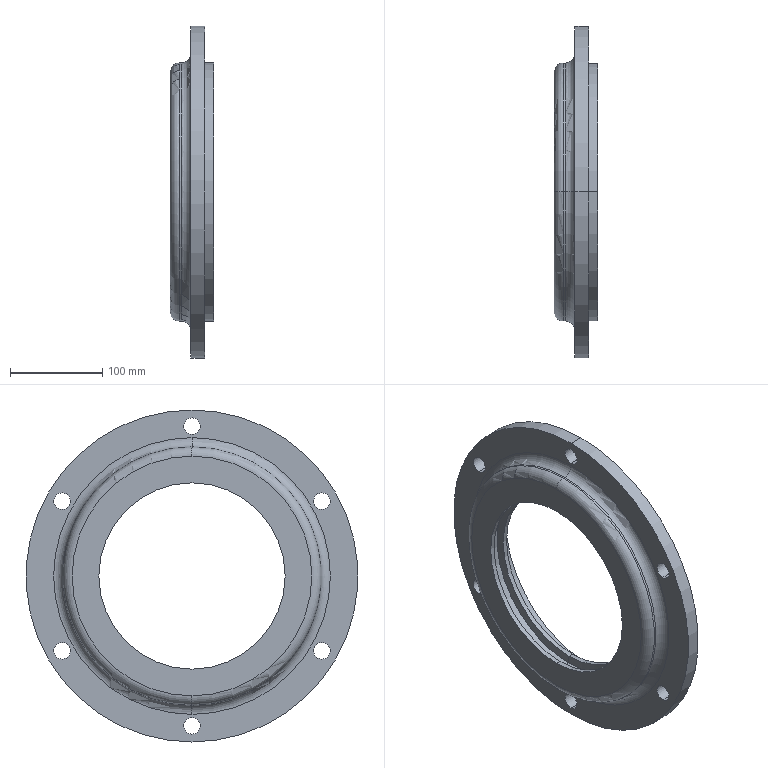Part | SolidWorks | features ICE 1, Revolution 1 | 1 solid | 41 faces | box 47.4 x 360 x 360 mm | volume 1531898 mm3 | cylinder 26 | torus 6 | plane 5 | cone 4 | commonest cylinder face diameters 18 x12 202 x4 280 x4 219 x2 250 x2 360 x2
STEP:
#1=CARTESIAN_POINT('',(9223.135,0.,159.026));
#2=VERTEX_POINT('',#1);
#3=CARTESIAN_POINT('',(9223.135,0.,141.026));
#4=VERTEX_POINT('',#3);
#5=CARTESIAN_POINT('',(9223.135,0.,150.026));
#6=DIRECTION('',(1.,0.,0.));
#7=DIRECTION('',(0.,0.,-1.));
#8=AXIS2_PLACEMENT_3D('',#5,#6,#7);
#9=CIRCLE('',#8,9.);
#10=EDGE_CURVE('',#2,#4,#9,.T.);
#11=ORIENTED_EDGE('',*,*,#10,.F.);
#12=CARTESIAN_POINT('',(9238.135,0.,159.026));
#13=VERTEX_POINT('',#12);
#14=CARTESIAN_POINT('',(9200.735,0.,159.026));
#15=DIRECTION('',(1.,0.,0.));
#16=VECTOR('',#15,1000.);
#17=LINE('',#14,#16);
#18=EDGE_CURVE('',#2,#13,#17,.T.);
#19=ORIENTED_EDGE('',*,*,#18,.T.);
#20=CARTESIAN_POINT('',(9238.135,0.,141.026));
#21=VERTEX_POINT('',#20);
#22=CARTESIAN_POINT('',(9238.135,0.,150.026));
#23=DIRECTION('',(1.,0.,0.));
#24=DIRECTION('',(0.,0.,-1.));
#25=AXIS2_PLACEMENT_3D('',#22,#23,#24);
#26=CIRCLE('',#25,9.);
#27=EDGE_CURVE('',#13,#21,#26,.T.);
#28=ORIENTED_EDGE('',*,*,#27,.T.);
#29=CARTESIAN_POINT('',(9200.735,0.,141.026));
#30=DIRECTION('',(1.,0.,0.));
#31=VECTOR('',#30,1000.);
#32=LINE('',#29,#31);
#33=EDGE_CURVE('',#4,#21,#32,.T.);
#34=ORIENTED_EDGE('',*,*,#33,.F.);
#35=EDGE_LOOP('',(#11,#19,#28,#34));
#36=FACE_OUTER_BOUND('',#35,.T.);
#37=CARTESIAN_POINT('',(9200.735,0.,150.026));
#38=DIRECTION('',(1.,0.,0.));
#39=DIRECTION('',(0.,0.,-1.));
#40=AXIS2_PLACEMENT_3D('',#37,#38,#39);
#41=CYLINDRICAL_SURFACE('',#40,9.);
#42=ADVANCED_FACE('',(#36),#41,.F.);
#43=CARTESIAN_POINT('',(9223.135,-140.729,77.776));
#44=VERTEX_POINT('',#43);
#45=CARTESIAN_POINT('',(9223.135,-140.729,59.776));
#46=VERTEX_POINT('',#45);
#47=CARTESIAN_POINT('',(9223.135,-140.729,68.776));
#48=DIRECTION('',(1.,0.,0.));
#49=DIRECTION('',(0.,0.,-1.));
#50=AXIS2_PLACEMENT_3D('',#47,#48,#49);
#51=CIRCLE('',#50,9.);
#52=EDGE_CURVE('',#44,#46,#51,.T.);
#53=ORIENTED_EDGE('',*,*,#52,.F.);
#54=CARTESIAN_POINT('',(9238.135,-140.729,77.776));
#55=VERTEX_POINT('',#54);
#56=CARTESIAN_POINT('',(9200.735,-140.729,77.776));
#57=DIRECTION('',(1.,0.,0.));
#58=VECTOR('',#57,1000.);
#59=LINE('',#56,#58);
#60=EDGE_CURVE('',#44,#55,#59,.T.);
#61=ORIENTED_EDGE('',*,*,#60,.T.);
#62=CARTESIAN_POINT('',(9238.135,-140.729,59.776));
#63=VERTEX_POINT('',#62);
#64=CARTESIAN_POINT('',(9238.135,-140.729,68.776));
#65=DIRECTION('',(1.,0.,0.));
#66=DIRECTION('',(0.,0.,-1.));
#67=AXIS2_PLACEMENT_3D('',#64,#65,#66);
#68=CIRCLE('',#67,9.);
#69=EDGE_CURVE('',#55,#63,#68,.T.);
#70=ORIENTED_EDGE('',*,*,#69,.T.);
#71=CARTESIAN_POINT('',(9200.735,-140.729,59.776));
#72=DIRECTION('',(1.,0.,0.));
#73=VECTOR('',#72,1000.);
#74=LINE('',#71,#73);
#75=EDGE_CURVE('',#46,#63,#74,.T.);
#76=ORIENTED_EDGE('',*,*,#75,.F.);
#77=EDGE_LOOP('',(#53,#61,#70,#76));
#78=FACE_OUTER_BOUND('',#77,.T.);
#79=CARTESIAN_POINT('',(9200.735,-140.729,68.776));
#80=DIRECTION('',(1.,0.,0.));
#81=DIRECTION('',(0.,0.,-1.));
#82=AXIS2_PLACEMENT_3D('',#79,#80,#81);
#83=CYLINDRICAL_SURFACE('',#82,9.);
#84=ADVANCED_FACE('',(#78),#83,.F.);
#85=CARTESIAN_POINT('',(9223.135,-140.729,-84.724));
#86=VERTEX_POINT('',#85);
#87=CARTESIAN_POINT('',(9223.135,-140.729,-102.724));
#88=VERTEX_POINT('',#87);
#89=CARTESIAN_POINT('',(9223.135,-140.729,-93.724));
#90=DIRECTION('',(1.,0.,0.));
#91=DIRECTION('',(0.,0.,-1.));
#92=AXIS2_PLACEMENT_3D('',#89,#90,#91);
#93=CIRCLE('',#92,9.);
#94=EDGE_CURVE('',#86,#88,#93,.T.);
#95=ORIENTED_EDGE('',*,*,#94,.F.);
#96=CARTESIAN_POINT('',(9238.135,-140.729,-84.724));
#97=VERTEX_POINT('',#96);
#98=CARTESIAN_POINT('',(9200.735,-140.729,-84.724));
#99=DIRECTION('',(1.,0.,0.));
#100=VECTOR('',#99,1000.);
#101=LINE('',#98,#100);
#102=EDGE_CURVE('',#86,#97,#101,.T.);
#103=ORIENTED_EDGE('',*,*,#102,.T.);
#104=CARTESIAN_POINT('',(9238.135,-140.729,-102.724));
#105=VERTEX_POINT('',#104);
#106=CARTESIAN_POINT('',(9238.135,-140.729,-93.724));
#107=DIRECTION('',(1.,0.,0.));
#108=DIRECTION('',(0.,0.,-1.));
#109=AXIS2_PLACEMENT_3D('',#106,#107,#108);
#110=CIRCLE('',#109,9.);
#111=EDGE_CURVE('',#97,#105,#110,.T.);
#112=ORIENTED_EDGE('',*,*,#111,.T.);
#113=CARTESIAN_POINT('',(9200.735,-140.729,-102.724));
#114=DIRECTION('',(1.,0.,0.));
#115=VECTOR('',#114,1000.);
#116=LINE('',#113,#115);
#117=EDGE_CURVE('',#88,#105,#116,.T.);
#118=ORIENTED_EDGE('',*,*,#117,.F.);
#119=EDGE_LOOP('',(#95,#103,#112,#118));
#120=FACE_OUTER_BOUND('',#119,.T.);
#121=CARTESIAN_POINT('',(9200.735,-140.729,-93.724));
#122=DIRECTION('',(1.,0.,0.));
#123=DIRECTION('',(0.,0.,-1.));
#124=AXIS2_PLACEMENT_3D('',#121,#122,#123);
#125=CYLINDRICAL_SURFACE('',#124,9.);
#126=ADVANCED_FACE('',(#120),#125,.F.);
#127=CARTESIAN_POINT('',(9223.135,0.,-165.974));
#128=VERTEX_POINT('',#127);
#129=CARTESIAN_POINT('',(9223.135,0.,-183.974));
#130=VERTEX_POINT('',#129);
#131=CARTESIAN_POINT('',(9223.135,0.,-174.974));
#132=DIRECTION('',(1.,0.,0.));
#133=DIRECTION('',(0.,0.,-1.));
#134=AXIS2_PLACEMENT_3D('',#131,#132,#133);
#135=CIRCLE('',#134,9.);
#136=EDGE_CURVE('',#128,#130,#135,.T.);
#137=ORIENTED_EDGE('',*,*,#136,.F.);
#138=CARTESIAN_POINT('',(9238.135,0.,-165.974));
#139=VERTEX_POINT('',#138);
#140=CARTESIAN_POINT('',(9200.735,0.,-165.974));
#141=DIRECTION('',(1.,0.,0.));
#142=VECTOR('',#141,1000.);
#143=LINE('',#140,#142);
#144=EDGE_CURVE('',#128,#139,#143,.T.);
#145=ORIENTED_EDGE('',*,*,#144,.T.);
#146=CARTESIAN_POINT('',(9238.135,0.,-183.974));
#147=VERTEX_POINT('',#146);
#148=CARTESIAN_POINT('',(9238.135,0.,-174.974));
#149=DIRECTION('',(1.,0.,0.));
#150=DIRECTION('',(0.,0.,-1.));
#151=AXIS2_PLACEMENT_3D('',#148,#149,#150);
#152=CIRCLE('',#151,9.);
#153=EDGE_CURVE('',#139,#147,#152,.T.);
#154=ORIENTED_EDGE('',*,*,#153,.T.);
#155=CARTESIAN_POINT('',(9200.735,0.,-183.974));
#156=DIRECTION('',(1.,0.,0.));
#157=VECTOR('',#156,1000.);
#158=LINE('',#155,#157);
#159=EDGE_CURVE('',#130,#147,#158,.T.);
#160=ORIENTED_EDGE('',*,*,#159,.F.);
#161=EDGE_LOOP('',(#137,#145,#154,#160));
#162=FACE_OUTER_BOUND('',#161,.T.);
#163=CARTESIAN_POINT('',(9200.735,0.,-174.974));
#164=DIRECTION('',(1.,0.,0.));
#165=DIRECTION('',(0.,0.,-1.));
#166=AXIS2_PLACEMENT_3D('',#163,#164,#165);
#167=CYLINDRICAL_SURFACE('',#166,9.);
#168=ADVANCED_FACE('',(#162),#167,.F.);
#169=CARTESIAN_POINT('',(9223.135,140.729,-84.724));
#170=VERTEX_POINT('',#169);
#171=CARTESIAN_POINT('',(9223.135,140.729,-102.724));
#172=VERTEX_POINT('',#171);
#173=CARTESIAN_POINT('',(9223.135,140.729,-93.724));
#174=DIRECTION('',(1.,0.,0.));
#175=DIRECTION('',(0.,0.,-1.));
#176=AXIS2_PLACEMENT_3D('',#173,#174,#175);
#177=CIRCLE('',#176,9.);
#178=EDGE_CURVE('',#170,#172,#177,.T.);
#179=ORIENTED_EDGE('',*,*,#178,.F.);
#180=CARTESIAN_POINT('',(9238.135,140.729,-84.724));
#181=VERTEX_POINT('',#180);
#182=CARTESIAN_POINT('',(9200.735,140.729,-84.724));
#183=DIRECTION('',(1.,0.,0.));
#184=VECTOR('',#183,1000.);
#185=LINE('',#182,#184);
#186=EDGE_CURVE('',#170,#181,#185,.T.);
#187=ORIENTED_EDGE('',*,*,#186,.T.);
#188=CARTESIAN_POINT('',(9238.135,140.729,-102.724));
#189=VERTEX_POINT('',#188);
#190=CARTESIAN_POINT('',(9238.135,140.729,-93.724));
#191=DIRECTION('',(1.,0.,0.));
#192=DIRECTION('',(0.,0.,-1.));
#193=AXIS2_PLACEMENT_3D('',#190,#191,#192);
#194=CIRCLE('',#193,9.);
#195=EDGE_CURVE('',#181,#189,#194,.T.);
#196=ORIENTED_EDGE('',*,*,#195,.T.);
#197=CARTESIAN_POINT('',(9200.735,140.729,-102.724));
#198=DIRECTION('',(1.,0.,0.));
#199=VECTOR('',#198,1000.);
#200=LINE('',#197,#199);
#201=EDGE_CURVE('',#172,#189,#200,.T.);
#202=ORIENTED_EDGE('',*,*,#201,.F.);
#203=EDGE_LOOP('',(#179,#187,#196,#202));
#204=FACE_OUTER_BOUND('',#203,.T.);
#205=CARTESIAN_POINT('',(9200.735,140.729,-93.724));
#206=DIRECTION('',(1.,0.,0.));
#207=DIRECTION('',(0.,0.,-1.));
#208=AXIS2_PLACEMENT_3D('',#205,#206,#207);
#209=CYLINDRICAL_SURFACE('',#208,9.);
#210=ADVANCED_FACE('',(#204),#209,.F.);
#211=CARTESIAN_POINT('',(9223.135,140.729,77.776));
#212=VERTEX_POINT('',#211);
#213=CARTESIAN_POINT('',(9223.135,140.729,59.776));
#214=VERTEX_POINT('',#213);
#215=CARTESIAN_POINT('',(9223.135,140.729,68.776));
#216=DIRECTION('',(1.,0.,0.));
#217=DIRECTION('',(0.,0.,-1.));
#218=AXIS2_PLACEMENT_3D('',#215,#216,#217);
#219=CIRCLE('',#218,9.);
#220=EDGE_CURVE('',#212,#214,#219,.T.);
#221=ORIENTED_EDGE('',*,*,#220,.F.);
#222=CARTESIAN_POINT('',(9238.135,140.729,77.776));
#223=VERTEX_POINT('',#222);
#224=CARTESIAN_POINT('',(9200.735,140.729,77.776));
#225=DIRECTION('',(1.,0.,0.));
#226=VECTOR('',#225,1000.);
#227=LINE('',#224,#226);
#228=EDGE_CURVE('',#212,#223,#227,.T.);
#229=ORIENTED_EDGE('',*,*,#228,.T.);
#230=CARTESIAN_POINT('',(9238.135,140.729,59.776));
#231=VERTEX_POINT('',#230);
#232=CARTESIAN_POINT('',(9238.135,140.729,68.776));
#233=DIRECTION('',(1.,0.,0.));
#234=DIRECTION('',(0.,0.,-1.));
#235=AXIS2_PLACEMENT_3D('',#232,#233,#234);
#236=CIRCLE('',#235,9.);
#237=EDGE_CURVE('',#223,#231,#236,.T.);
#238=ORIENTED_EDGE('',*,*,#237,.T.);
#239=CARTESIAN_POINT('',(9200.735,140.729,59.776));
#240=DIRECTION('',(1.,0.,0.));
#241=VECTOR('',#240,1000.);
#242=LINE('',#239,#241);
#243=EDGE_CURVE('',#214,#231,#242,.T.);
#244=ORIENTED_EDGE('',*,*,#243,.F.);
#245=EDGE_LOOP('',(#221,#229,#238,#244));
#246=FACE_OUTER_BOUND('',#245,.T.);
#247=CARTESIAN_POINT('',(9200.735,140.729,68.776));
#248=DIRECTION('',(1.,0.,0.));
#249=DIRECTION('',(0.,0.,-1.));
#250=AXIS2_PLACEMENT_3D('',#247,#248,#249);
#251=CYLINDRICAL_SURFACE('',#250,9.);
#252=ADVANCED_FACE('',(#246),#251,.F.);
#253=CARTESIAN_POINT('',(9225.135,0.,-113.474));
#254=VERTEX_POINT('',#253);
#255=CARTESIAN_POINT('',(9225.135,0.,88.526));
#256=VERTEX_POINT('',#255);
#257=CARTESIAN_POINT('',(9225.135,0.,-12.474));
#258=DIRECTION('',(-1.,0.,0.));
#259=DIRECTION('',(0.,0.,1.));
#260=AXIS2_PLACEMENT_3D('',#257,#258,#259);
#261=CIRCLE('',#260,101.);
#262=EDGE_CURVE('',#254,#256,#261,.T.);
#263=ORIENTED_EDGE('',*,*,#262,.F.);
#264=CARTESIAN_POINT('',(9219.979,0.,-113.474));
#265=VERTEX_POINT('',#264);
#266=CARTESIAN_POINT('',(9092.87,0.,-113.474));
#267=DIRECTION('',(-1.,0.,0.));
#268=VECTOR('',#267,1000.);
#269=LINE('',#266,#268);
#270=EDGE_CURVE('',#254,#265,#269,.T.);
#271=ORIENTED_EDGE('',*,*,#270,.T.);
#272=CARTESIAN_POINT('',(9219.979,0.,88.526));
#273=VERTEX_POINT('',#272);
#274=CARTESIAN_POINT('',(9219.979,0.,-12.474));
#275=DIRECTION('',(-1.,0.,0.));
#276=DIRECTION('',(0.,0.,1.));
#277=AXIS2_PLACEMENT_3D('',#274,#275,#276);
#278=CIRCLE('',#277,101.);
#279=EDGE_CURVE('',#265,#273,#278,.T.);
#280=ORIENTED_EDGE('',*,*,#279,.T.);
#281=CARTESIAN_POINT('',(9092.87,0.,88.526));
#282=DIRECTION('',(-1.,0.,0.));
#283=VECTOR('',#282,1000.);
#284=LINE('',#281,#283);
#285=EDGE_CURVE('',#256,#273,#284,.T.);
#286=ORIENTED_EDGE('',*,*,#285,.F.);
#287=EDGE_LOOP('',(#263,#271,#280,#286));
#288=FACE_OUTER_BOUND('',#287,.T.);
#289=CARTESIAN_POINT('',(9092.87,0.,-12.474));
#290=DIRECTION('',(-1.,0.,0.));
#291=DIRECTION('',(0.,0.,1.));
#292=AXIS2_PLACEMENT_3D('',#289,#290,#291);
#293=CYLINDRICAL_SURFACE('',#292,101.);
#294=ADVANCED_FACE('',(#288),#293,.F.);
#295=ORIENTED_EDGE('',*,*,#279,.F.);
#296=CARTESIAN_POINT('',(9218.935,0.,-121.974));
#297=VERTEX_POINT('',#296);
#298=CARTESIAN_POINT('',(9218.935,0.,-121.974));
#299=DIRECTION('',(-0.1219,0.,-0.9925));
#300=VECTOR('',#299,1000.);
#301=LINE('',#298,#300);
#302=EDGE_CURVE('',#265,#297,#301,.T.);
#303=ORIENTED_EDGE('',*,*,#302,.T.);
#304=CARTESIAN_POINT('',(9218.935,0.,97.026));
#305=VERTEX_POINT('',#304);
#306=CARTESIAN_POINT('',(9218.935,0.,-12.474));
#307=DIRECTION('',(-1.,0.,0.));
#308=DIRECTION('',(0.,0.,1.));
#309=AXIS2_PLACEMENT_3D('',#306,#307,#308);
#310=CIRCLE('',#309,109.5);
#311=EDGE_CURVE('',#297,#305,#310,.T.);
#312=ORIENTED_EDGE('',*,*,#311,.T.);
#313=CARTESIAN_POINT('',(9218.935,0.,97.026));
#314=DIRECTION('',(-0.1219,0.,0.9925));
#315=VECTOR('',#314,1000.);
#316=LINE('',#313,#315);
#317=EDGE_CURVE('',#273,#305,#316,.T.);
#318=ORIENTED_EDGE('',*,*,#317,.F.);
#319=EDGE_LOOP('',(#295,#303,#312,#318));
#320=FACE_OUTER_BOUND('',#319,.T.);
#321=CARTESIAN_POINT('',(9218.935,0.,-12.474));
#322=DIRECTION('',(-1.,0.,0.));
#323=DIRECTION('',(0.,0.,1.));
#324=AXIS2_PLACEMENT_3D('',#321,#322,#323);
#325=CONICAL_SURFACE('',#324,109.5,1.449);
#326=ADVANCED_FACE('',(#320),#325,.F.);
#327=ORIENTED_EDGE('',*,*,#311,.F.);
#328=CARTESIAN_POINT('',(9206.935,0.,-121.974));
#329=VERTEX_POINT('',#328);
#330=CARTESIAN_POINT('',(9092.87,0.,-121.974));
#331=DIRECTION('',(-1.,0.,0.));
#332=VECTOR('',#331,1000.);
#333=LINE('',#330,#332);
#334=EDGE_CURVE('',#297,#329,#333,.T.);
#335=ORIENTED_EDGE('',*,*,#334,.T.);
#336=CARTESIAN_POINT('',(9206.935,0.,97.026));
#337=VERTEX_POINT('',#336);
#338=CARTESIAN_POINT('',(9206.935,0.,-12.474));
#339=DIRECTION('',(-1.,0.,0.));
#340=DIRECTION('',(0.,0.,1.));
#341=AXIS2_PLACEMENT_3D('',#338,#339,#340);
#342=CIRCLE('',#341,109.5);
#343=EDGE_CURVE('',#329,#337,#342,.T.);
#344=ORIENTED_EDGE('',*,*,#343,.T.);
#345=CARTESIAN_POINT('',(9092.87,0.,97.026));
#346=DIRECTION('',(-1.,0.,0.));
#347=VECTOR('',#346,1000.);
#348=LINE('',#345,#347);
#349=EDGE_CURVE('',#305,#337,#348,.T.);
#350=ORIENTED_EDGE('',*,*,#349,.F.);
#351=EDGE_LOOP('',(#327,#335,#344,#350));
#352=FACE_OUTER_BOUND('',#351,.T.);
#353=CARTESIAN_POINT('',(9092.87,0.,-12.474));
#354=DIRECTION('',(-1.,0.,0.));
#355=DIRECTION('',(0.,0.,1.));
#356=AXIS2_PLACEMENT_3D('',#353,#354,#355);
#357=CYLINDRICAL_SURFACE('',#356,109.5);
#358=ADVANCED_FACE('',(#352),#357,.F.);
#359=CARTESIAN_POINT('',(9205.892,0.,-113.474));
#360=VERTEX_POINT('',#359);
#361=CARTESIAN_POINT('',(9205.892,0.,88.526));
#362=VERTEX_POINT('',#361);
#363=CARTESIAN_POINT('',(9205.892,0.,-12.474));
#364=DIRECTION('',(-1.,0.,0.));
#365=DIRECTION('',(0.,0.,1.));
#366=AXIS2_PLACEMENT_3D('',#363,#364,#365);
#367=CIRCLE('',#366,101.);
#368=EDGE_CURVE('',#360,#362,#367,.T.);
#369=ORIENTED_EDGE('',*,*,#368,.T.);
#370=CARTESIAN_POINT('',(9206.935,0.,97.026));
#371=DIRECTION('',(0.1219,0.,0.9925));
#372=VECTOR('',#371,1000.);
#373=LINE('',#370,#372);
#374=EDGE_CURVE('',#362,#337,#373,.T.);
#375=ORIENTED_EDGE('',*,*,#374,.T.);
#376=ORIENTED_EDGE('',*,*,#343,.F.);
#377=CARTESIAN_POINT('',(9206.935,0.,-121.974));
#378=DIRECTION('',(0.1219,0.,-0.9925));
#379=VECTOR('',#378,1000.);
#380=LINE('',#377,#379);
#381=EDGE_CURVE('',#360,#329,#380,.T.);
#382=ORIENTED_EDGE('',*,*,#381,.F.);
#383=EDGE_LOOP('',(#369,#375,#376,#382));
#384=FACE_OUTER_BOUND('',#383,.T.);
#385=CARTESIAN_POINT('',(9206.935,0.,-12.474));
#386=DIRECTION('',(1.,0.,0.));
#387=DIRECTION('',(0.,0.,-1.));
#388=AXIS2_PLACEMENT_3D('',#385,#386,#387);
#389=CONICAL_SURFACE('',#388,109.5,1.449);
#390=ADVANCED_FACE('',(#384),#389,.F.);
#391=ORIENTED_EDGE('',*,*,#368,.F.);
#392=CARTESIAN_POINT('',(9200.735,0.,-113.474));
#393=VERTEX_POINT('',#392);
#394=CARTESIAN_POINT('',(9092.87,0.,-113.474));
#395=DIRECTION('',(-1.,0.,0.));
#396=VECTOR('',#395,1000.);
#397=LINE('',#394,#396);
#398=EDGE_CURVE('',#360,#393,#397,.T.);
#399=ORIENTED_EDGE('',*,*,#398,.T.);
#400=CARTESIAN_POINT('',(9200.735,0.,88.526));
#401=VERTEX_POINT('',#400);
#402=CARTESIAN_POINT('',(9200.735,0.,-12.474));
#403=DIRECTION('',(-1.,0.,0.));
#404=DIRECTION('',(0.,0.,1.));
#405=AXIS2_PLACEMENT_3D('',#402,#403,#404);
#406=CIRCLE('',#405,101.);
#407=EDGE_CURVE('',#393,#401,#406,.T.);
#408=ORIENTED_EDGE('',*,*,#407,.T.);
#409=CARTESIAN_POINT('',(9092.87,0.,88.526));
#410=DIRECTION('',(-1.,0.,0.));
#411=VECTOR('',#410,1000.);
#412=LINE('',#409,#411);
#413=EDGE_CURVE('',#362,#401,#412,.T.);
#414=ORIENTED_EDGE('',*,*,#413,.F.);
#415=EDGE_LOOP('',(#391,#399,#408,#414));
#416=FACE_OUTER_BOUND('',#415,.T.);
#417=CARTESIAN_POINT('',(9092.87,0.,-12.474));
#418=DIRECTION('',(-1.,0.,0.));
#419=DIRECTION('',(0.,0.,1.));
#420=AXIS2_PLACEMENT_3D('',#417,#418,#419);
#421=CYLINDRICAL_SURFACE('',#420,101.);
#422=ADVANCED_FACE('',(#416),#421,.F.);
#423=CARTESIAN_POINT('',(9210.735,0.,127.526));
#424=VERTEX_POINT('',#423);
#425=CARTESIAN_POINT('',(9210.735,0.,-152.474));
#426=VERTEX_POINT('',#425);
#427=CARTESIAN_POINT('',(9210.735,0.,-12.474));
#428=DIRECTION('',(-1.,0.,0.));
#429=DIRECTION('',(0.,0.,1.));
#430=AXIS2_PLACEMENT_3D('',#427,#428,#429);
#431=CIRCLE('',#430,140.);
#432=EDGE_CURVE('',#424,#426,#431,.T.);
#433=ORIENTED_EDGE('',*,*,#432,.T.);
#434=CARTESIAN_POINT('',(9200.735,0.,-142.474));
#435=VERTEX_POINT('',#434);
#436=CARTESIAN_POINT('',(9210.735,0.,-142.474));
#437=DIRECTION('',(0.,1.,0.));
#438=DIRECTION('',(0.,0.,1.));
#439=AXIS2_PLACEMENT_3D('',#436,#437,#438);
#440=CIRCLE('',#439,10.);
#441=EDGE_CURVE('',#426,#435,#440,.T.);
#442=ORIENTED_EDGE('',*,*,#441,.T.);
#443=CARTESIAN_POINT('',(9200.735,0.,117.526));
#444=VERTEX_POINT('',#443);
#445=CARTESIAN_POINT('',(9200.735,0.,-12.474));
#446=DIRECTION('',(-1.,0.,0.));
#447=DIRECTION('',(0.,0.,1.));
#448=AXIS2_PLACEMENT_3D('',#445,#446,#447);
#449=CIRCLE('',#448,130.);
#450=EDGE_CURVE('',#444,#435,#449,.T.);
#451=ORIENTED_EDGE('',*,*,#450,.F.);
#452=CARTESIAN_POINT('',(9210.735,0.,117.526));
#453=DIRECTION('',(0.,-1.,0.));
#454=DIRECTION('',(0.,0.,-1.));
#455=AXIS2_PLACEMENT_3D('',#452,#453,#454);
#456=CIRCLE('',#455,10.);
#457=EDGE_CURVE('',#424,#444,#456,.T.);
#458=ORIENTED_EDGE('',*,*,#457,.F.);
#459=EDGE_LOOP('',(#433,#442,#451,#458));
#460=FACE_OUTER_BOUND('',#459,.T.);
#461=CARTESIAN_POINT('',(9210.735,0.,-12.474));
#462=DIRECTION('',(-1.,0.,0.));
#463=DIRECTION('',(0.,0.,1.));
#464=AXIS2_PLACEMENT_3D('',#461,#462,#463);
#465=TOROIDAL_SURFACE('',#464,130.,10.);
#466=ADVANCED_FACE('',(#460),#465,.T.);
#467=CARTESIAN_POINT('',(9213.135,0.,127.526));
#468=VERTEX_POINT('',#467);
#469=CARTESIAN_POINT('',(9213.135,0.,-152.474));
#470=VERTEX_POINT('',#469);
#471=CARTESIAN_POINT('',(9213.135,0.,-12.474));
#472=DIRECTION('',(-1.,0.,0.));
#473=DIRECTION('',(0.,0.,1.));
#474=AXIS2_PLACEMENT_3D('',#471,#472,#473);
#475=CIRCLE('',#474,140.);
#476=EDGE_CURVE('',#468,#470,#475,.T.);
#477=ORIENTED_EDGE('',*,*,#476,.T.);
#478=CARTESIAN_POINT('',(9092.87,0.,-152.474));
#479=DIRECTION('',(-1.,0.,0.));
#480=VECTOR('',#479,1000.);
#481=LINE('',#478,#480);
#482=EDGE_CURVE('',#470,#426,#481,.T.);
#483=ORIENTED_EDGE('',*,*,#482,.T.);
#484=ORIENTED_EDGE('',*,*,#432,.F.);
#485=CARTESIAN_POINT('',(9092.87,0.,127.526));
#486=DIRECTION('',(-1.,0.,0.));
#487=VECTOR('',#486,1000.);
#488=LINE('',#485,#487);
#489=EDGE_CURVE('',#468,#424,#488,.T.);
#490=ORIENTED_EDGE('',*,*,#489,.F.);
#491=EDGE_LOOP('',(#477,#483,#484,#490));
#492=FACE_OUTER_BOUND('',#491,.T.);
#493=CARTESIAN_POINT('',(9092.87,0.,-12.474));
#494=DIRECTION('',(-1.,0.,0.));
#495=DIRECTION('',(0.,0.,1.));
#496=AXIS2_PLACEMENT_3D('',#493,#494,#495);
#497=CYLINDRICAL_SURFACE('',#496,140.);
#498=ADVANCED_FACE('',(#492),#497,.T.);
#499=CARTESIAN_POINT('',(9213.135,0.,-12.474));
#500=DIRECTION('',(-1.,0.,0.));
#501=DIRECTION('',(0.,0.,1.));
#502=AXIS2_PLACEMENT_3D('',#499,#500,#501);
#503=CIRCLE('',#502,140.);
#504=EDGE_CURVE('',#470,#468,#503,.T.);
#505=ORIENTED_EDGE('',*,*,#504,.F.);
#506=CARTESIAN_POINT('',(9223.135,0.,-162.474));
#507=VERTEX_POINT('',#506);
#508=CARTESIAN_POINT('',(9213.135,0.,-162.474));
#509=DIRECTION('',(0.,1.,0.));
#510=DIRECTION('',(0.,0.,1.));
#511=AXIS2_PLACEMENT_3D('',#508,#509,#510);
#512=CIRCLE('',#511,10.);
#513=EDGE_CURVE('',#470,#507,#512,.T.);
#514=ORIENTED_EDGE('',*,*,#513,.T.);
#515=CARTESIAN_POINT('',(9223.135,0.,137.526));
#516=VERTEX_POINT('',#515);
#517=CARTESIAN_POINT('',(9223.135,0.,-12.474));
#518=DIRECTION('',(-1.,0.,0.));
#519=DIRECTION('',(0.,0.,1.));
#520=AXIS2_PLACEMENT_3D('',#517,#518,#519);
#521=CIRCLE('',#520,150.);
#522=EDGE_CURVE('',#507,#516,#521,.T.);
#523=ORIENTED_EDGE('',*,*,#522,.T.);
#524=CARTESIAN_POINT('',(9213.135,0.,137.526));
#525=DIRECTION('',(0.,-1.,0.));
#526=DIRECTION('',(0.,0.,-1.));
#527=AXIS2_PLACEMENT_3D('',#524,#525,#526);
#528=CIRCLE('',#527,10.);
#529=EDGE_CURVE('',#468,#516,#528,.T.);
#530=ORIENTED_EDGE('',*,*,#529,.F.);
#531=EDGE_LOOP('',(#505,#514,#523,#530));
#532=FACE_OUTER_BOUND('',#531,.T.);
#533=CARTESIAN_POINT('',(9213.135,0.,-12.474));
#534=DIRECTION('',(-1.,0.,0.));
#535=DIRECTION('',(0.,0.,1.));
#536=AXIS2_PLACEMENT_3D('',#533,#534,#535);
#537=TOROIDAL_SURFACE('',#536,150.,10.);
#538=ADVANCED_FACE('',(#532),#537,.F.);
#539=CARTESIAN_POINT('',(9238.135,0.,167.526));
#540=VERTEX_POINT('',#539);
#541=CARTESIAN_POINT('',(9238.135,0.,-192.474));
#542=VERTEX_POINT('',#541);
#543=CARTESIAN_POINT('',(9238.135,0.,-12.474));
#544=DIRECTION('',(-1.,0.,0.));
#545=DIRECTION('',(0.,0.,1.));
#546=AXIS2_PLACEMENT_3D('',#543,#544,#545);
#547=CIRCLE('',#546,180.);
#548=EDGE_CURVE('',#540,#542,#547,.T.);
#549=ORIENTED_EDGE('',*,*,#548,.T.);
#550=CARTESIAN_POINT('',(9223.135,0.,-192.474));
#551=VERTEX_POINT('',#550);
#552=CARTESIAN_POINT('',(9092.87,0.,-192.474));
#553=DIRECTION('',(-1.,0.,0.));
#554=VECTOR('',#553,1000.);
#555=LINE('',#552,#554);
#556=EDGE_CURVE('',#542,#551,#555,.T.);
#557=ORIENTED_EDGE('',*,*,#556,.T.);
#558=CARTESIAN_POINT('',(9223.135,0.,167.526));
#559=VERTEX_POINT('',#558);
#560=CARTESIAN_POINT('',(9223.135,0.,-12.474));
#561=DIRECTION('',(-1.,0.,0.));
#562=DIRECTION('',(0.,0.,1.));
#563=AXIS2_PLACEMENT_3D('',#560,#561,#562);
#564=CIRCLE('',#563,180.);
#565=EDGE_CURVE('',#559,#551,#564,.T.);
#566=ORIENTED_EDGE('',*,*,#565,.F.);
#567=CARTESIAN_POINT('',(9092.87,0.,167.526));
#568=DIRECTION('',(-1.,0.,0.));
#569=VECTOR('',#568,1000.);
#570=LINE('',#567,#569);
#571=EDGE_CURVE('',#540,#559,#570,.T.);
#572=ORIENTED_EDGE('',*,*,#571,.F.);
#573=EDGE_LOOP('',(#549,#557,#566,#572));
#574=FACE_OUTER_BOUND('',#573,.T.);
#575=CARTESIAN_POINT('',(9092.87,0.,-12.474));
#576=DIRECTION('',(-1.,0.,0.));
#577=DIRECTION('',(0.,0.,1.));
#578=AXIS2_PLACEMENT_3D('',#575,#576,#577);
#579=CYLINDRICAL_SURFACE('',#578,180.);
#580=ADVANCED_FACE('',(#574),#579,.T.);
#581=CARTESIAN_POINT('',(9248.135,0.,127.526));
#582=VERTEX_POINT('',#581);
#583=CARTESIAN_POINT('',(9248.135,0.,-152.474));
#584=VERTEX_POINT('',#583);
#585=CARTESIAN_POINT('',(9248.135,0.,-12.474));
#586=DIRECTION('',(-1.,0.,0.));
#587=DIRECTION('',(0.,0.,1.));
#588=AXIS2_PLACEMENT_3D('',#585,#586,#587);
#589=CIRCLE('',#588,140.);
#590=EDGE_CURVE('',#582,#584,#589,.T.);
#591=ORIENTED_EDGE('',*,*,#590,.T.);
#592=CARTESIAN_POINT('',(9238.135,0.,-152.474));
#593=VERTEX_POINT('',#592);
#594=CARTESIAN_POINT('',(9092.87,0.,-152.474));
#595=DIRECTION('',(-1.,0.,0.));
#596=VECTOR('',#595,1000.);
#597=LINE('',#594,#596);
#598=EDGE_CURVE('',#584,#593,#597,.T.);
#599=ORIENTED_EDGE('',*,*,#598,.T.);
#600=CARTESIAN_POINT('',(9238.135,0.,127.526));
#601=VERTEX_POINT('',#600);
#602=CARTESIAN_POINT('',(9238.135,0.,-12.474));
#603=DIRECTION('',(-1.,0.,0.));
#604=DIRECTION('',(0.,0.,1.));
#605=AXIS2_PLACEMENT_3D('',#602,#603,#604);
#606=CIRCLE('',#605,140.);
#607=EDGE_CURVE('',#601,#593,#606,.T.);
#608=ORIENTED_EDGE('',*,*,#607,.F.);
#609=CARTESIAN_POINT('',(9092.87,0.,127.526));
#610=DIRECTION('',(-1.,0.,0.));
#611=VECTOR('',#610,1000.);
#612=LINE('',#609,#611);
#613=EDGE_CURVE('',#582,#601,#612,.T.);
#614=ORIENTED_EDGE('',*,*,#613,.F.);
#615=EDGE_LOOP('',(#591,#599,#608,#614));
#616=FACE_OUTER_BOUND('',#615,.T.);
#617=CARTESIAN_POINT('',(9092.87,0.,-12.474));
#618=DIRECTION('',(-1.,0.,0.));
#619=DIRECTION('',(0.,0.,1.));
#620=AXIS2_PLACEMENT_3D('',#617,#618,#619);
#621=CYLINDRICAL_SURFACE('',#620,140.);
#622=ADVANCED_FACE('',(#616),#621,.T.);
#623=CARTESIAN_POINT('',(9248.135,0.,-137.474));
#624=VERTEX_POINT('',#623);
#625=CARTESIAN_POINT('',(9248.135,0.,112.526));
#626=VERTEX_POINT('',#625);
#627=CARTESIAN_POINT('',(9248.135,0.,-12.474));
#628=DIRECTION('',(-1.,0.,0.));
#629=DIRECTION('',(0.,0.,1.));
#630=AXIS2_PLACEMENT_3D('',#627,#628,#629);
#631=CIRCLE('',#630,125.);
#632=EDGE_CURVE('',#624,#626,#631,.T.);
#633=ORIENTED_EDGE('',*,*,#632,.F.);
#634=CARTESIAN_POINT('',(9235.135,0.,-137.474));
#635=VERTEX_POINT('',#634);
#636=CARTESIAN_POINT('',(9092.87,0.,-137.474));
#637=DIRECTION('',(-1.,0.,0.));
#638=VECTOR('',#637,1000.);
#639=LINE('',#636,#638);
#640=EDGE_CURVE('',#624,#635,#639,.T.);
#641=ORIENTED_EDGE('',*,*,#640,.T.);
#642=CARTESIAN_POINT('',(9235.135,0.,112.526));
#643=VERTEX_POINT('',#642);
#644=CARTESIAN_POINT('',(9235.135,0.,-12.474));
#645=DIRECTION('',(-1.,0.,0.));
#646=DIRECTION('',(0.,0.,1.));
#647=AXIS2_PLACEMENT_3D('',#644,#645,#646);
#648=CIRCLE('',#647,125.);
#649=EDGE_CURVE('',#635,#643,#648,.T.);
#650=ORIENTED_EDGE('',*,*,#649,.T.);
#651=CARTESIAN_POINT('',(9092.87,0.,112.526));
#652=DIRECTION('',(-1.,0.,0.));
#653=VECTOR('',#652,1000.);
#654=LINE('',#651,#653);
#655=EDGE_CURVE('',#626,#643,#654,.T.);
#656=ORIENTED_EDGE('',*,*,#655,.F.);
#657=EDGE_LOOP('',(#633,#641,#650,#656));
#658=FACE_OUTER_BOUND('',#657,.T.);
#659=CARTESIAN_POINT('',(9092.87,0.,-12.474));
#660=DIRECTION('',(-1.,0.,0.));
#661=DIRECTION('',(0.,0.,1.));
#662=AXIS2_PLACEMENT_3D('',#659,#660,#661);
#663=CYLINDRICAL_SURFACE('',#662,125.);
#664=ADVANCED_FACE('',(#658),#663,.F.);
#665=ORIENTED_EDGE('',*,*,#649,.F.);
#666=CARTESIAN_POINT('',(9225.135,0.,-127.474));
#667=VERTEX_POINT('',#666);
#668=CARTESIAN_POINT('',(9235.135,0.,-127.474));
#669=DIRECTION('',(0.,1.,0.));
#670=DIRECTION('',(0.,0.,1.));
#671=AXIS2_PLACEMENT_3D('',#668,#669,#670);
#672=CIRCLE('',#671,10.);
#673=EDGE_CURVE('',#635,#667,#672,.T.);
#674=ORIENTED_EDGE('',*,*,#673,.T.);
#675=CARTESIAN_POINT('',(9225.135,0.,102.526));
#676=VERTEX_POINT('',#675);
#677=CARTESIAN_POINT('',(9225.135,0.,-12.474));
#678=DIRECTION('',(-1.,0.,0.));
#679=DIRECTION('',(0.,0.,1.));
#680=AXIS2_PLACEMENT_3D('',#677,#678,#679);
#681=CIRCLE('',#680,115.);
#682=EDGE_CURVE('',#667,#676,#681,.T.);
#683=ORIENTED_EDGE('',*,*,#682,.T.);
#684=CARTESIAN_POINT('',(9235.135,0.,102.526));
#685=DIRECTION('',(0.,-1.,0.));
#686=DIRECTION('',(0.,0.,-1.));
#687=AXIS2_PLACEMENT_3D('',#684,#685,#686);
#688=CIRCLE('',#687,10.);
#689=EDGE_CURVE('',#643,#676,#688,.T.);
#690=ORIENTED_EDGE('',*,*,#689,.F.);
#691=EDGE_LOOP('',(#665,#674,#683,#690));
#692=FACE_OUTER_BOUND('',#691,.T.);
#693=CARTESIAN_POINT('',(9235.135,0.,-12.474));
#694=DIRECTION('',(-1.,0.,0.));
#695=DIRECTION('',(0.,0.,1.));
#696=AXIS2_PLACEMENT_3D('',#693,#694,#695);
#697=TOROIDAL_SURFACE('',#696,115.,10.);
#698=ADVANCED_FACE('',(#692),#697,.F.);
#699=ORIENTED_EDGE('',*,*,#673,.F.);
#700=CARTESIAN_POINT('',(9235.135,0.,-12.474));
#701=DIRECTION('',(-1.,0.,0.));
#702=DIRECTION('',(0.,0.,1.));
#703=AXIS2_PLACEMENT_3D('',#700,#701,#702);
#704=CIRCLE('',#703,125.);
#705=EDGE_CURVE('',#643,#635,#704,.T.);
#706=ORIENTED_EDGE('',*,*,#705,.F.);
#707=ORIENTED_EDGE('',*,*,#689,.T.);
#708=CARTESIAN_POINT('',(9225.135,0.,-12.474));
#709=DIRECTION('',(-1.,0.,0.));
#710=DIRECTION('',(0.,0.,1.));
#711=AXIS2_PLACEMENT_3D('',#708,#709,#710);
#712=CIRCLE('',#711,115.);
#713=EDGE_CURVE('',#676,#667,#712,.T.);
#714=ORIENTED_EDGE('',*,*,#713,.T.);
#715=EDGE_LOOP('',(#699,#706,#707,#714));
#716=FACE_OUTER_BOUND('',#715,.T.);
#717=CARTESIAN_POINT('',(9235.135,0.,-12.474));
#718=DIRECTION('',(-1.,0.,0.));
#719=DIRECTION('',(0.,0.,1.));
#720=AXIS2_PLACEMENT_3D('',#717,#718,#719);
#721=TOROIDAL_SURFACE('',#720,115.,10.);
#722=ADVANCED_FACE('',(#716),#721,.F.);
#723=ORIENTED_EDGE('',*,*,#640,.F.);
#724=CARTESIAN_POINT('',(9248.135,0.,-12.474));
#725=DIRECTION('',(-1.,0.,0.));
#726=DIRECTION('',(0.,0.,1.));
#727=AXIS2_PLACEMENT_3D('',#724,#725,#726);
#728=CIRCLE('',#727,125.);
#729=EDGE_CURVE('',#626,#624,#728,.T.);
#730=ORIENTED_EDGE('',*,*,#729,.F.);
#731=ORIENTED_EDGE('',*,*,#655,.T.);
#732=ORIENTED_EDGE('',*,*,#705,.T.);
#733=EDGE_LOOP('',(#723,#730,#731,#732));
#734=FACE_OUTER_BOUND('',#733,.T.);
#735=CARTESIAN_POINT('',(9092.87,0.,-12.474));
#736=DIRECTION('',(-1.,0.,0.));
#737=DIRECTION('',(0.,0.,1.));
#738=AXIS2_PLACEMENT_3D('',#735,#736,#737);
#739=CYLINDRICAL_SURFACE('',#738,125.);
#740=ADVANCED_FACE('',(#734),#739,.F.);
#741=ORIENTED_EDGE('',*,*,#729,.T.);
#742=ORIENTED_EDGE('',*,*,#632,.T.);
#743=EDGE_LOOP('',(#741,#742));
#744=FACE_BOUND('',#743,.T.);
#745=ORIENTED_EDGE('',*,*,#590,.F.);
#746=CARTESIAN_POINT('',(9248.135,0.,-12.474));
#747=DIRECTION('',(-1.,0.,0.));
#748=DIRECTION('',(0.,0.,1.));
#749=AXIS2_PLACEMENT_3D('',#746,#747,#748);
#750=CIRCLE('',#749,140.);
#751=EDGE_CURVE('',#584,#582,#750,.T.);
#752=ORIENTED_EDGE('',*,*,#751,.F.);
#753=EDGE_LOOP('',(#745,#752));
#754=FACE_OUTER_BOUND('',#753,.T.);
#755=CARTESIAN_POINT('',(9248.135,0.,0.));
#756=DIRECTION('',(1.,0.,0.));
#757=DIRECTION('',(0.,0.,-1.));
#758=AXIS2_PLACEMENT_3D('',#755,#756,#757);
#759=PLANE('',#758);
#760=ADVANCED_FACE('',(#744,#754),#759,.T.);
#761=ORIENTED_EDGE('',*,*,#598,.F.);
#762=ORIENTED_EDGE('',*,*,#751,.T.);
#763=ORIENTED_EDGE('',*,*,#613,.T.);
#764=CARTESIAN_POINT('',(9238.135,0.,-12.474));
#765=DIRECTION('',(-1.,0.,0.));
#766=DIRECTION('',(0.,0.,1.));
#767=AXIS2_PLACEMENT_3D('',#764,#765,#766);
#768=CIRCLE('',#767,140.);
#769=EDGE_CURVE('',#593,#601,#768,.T.);
#770=ORIENTED_EDGE('',*,*,#769,.F.);
#771=EDGE_LOOP('',(#761,#762,#763,#770));
#772=FACE_OUTER_BOUND('',#771,.T.);
#773=CARTESIAN_POINT('',(9092.87,0.,-12.474));
#774=DIRECTION('',(-1.,0.,0.));
#775=DIRECTION('',(0.,0.,1.));
#776=AXIS2_PLACEMENT_3D('',#773,#774,#775);
#777=CYLINDRICAL_SURFACE('',#776,140.);
#778=ADVANCED_FACE('',(#772),#777,.T.);
#779=CARTESIAN_POINT('',(9238.135,0.,150.026));
#780=DIRECTION('',(1.,0.,0.));
#781=DIRECTION('',(0.,0.,-1.));
#782=AXIS2_PLACEMENT_3D('',#779,#780,#781);
#783=CIRCLE('',#782,9.);
#784=EDGE_CURVE('',#21,#13,#783,.T.);
#785=ORIENTED_EDGE('',*,*,#784,.F.);
#786=ORIENTED_EDGE('',*,*,#27,.F.);
#787=EDGE_LOOP('',(#785,#786));
#788=FACE_BOUND('',#787,.T.);
#789=CARTESIAN_POINT('',(9238.135,-140.729,68.776));
#790=DIRECTION('',(1.,0.,0.));
#791=DIRECTION('',(0.,0.,-1.));
#792=AXIS2_PLACEMENT_3D('',#789,#790,#791);
#793=CIRCLE('',#792,9.);
#794=EDGE_CURVE('',#63,#55,#793,.T.);
#795=ORIENTED_EDGE('',*,*,#794,.F.);
#796=ORIENTED_EDGE('',*,*,#69,.F.);
#797=EDGE_LOOP('',(#795,#796));
#798=FACE_BOUND('',#797,.T.);
#799=CARTESIAN_POINT('',(9238.135,-140.729,-93.724));
#800=DIRECTION('',(1.,0.,0.));
#801=DIRECTION('',(0.,0.,-1.));
#802=AXIS2_PLACEMENT_3D('',#799,#800,#801);
#803=CIRCLE('',#802,9.);
#804=EDGE_CURVE('',#105,#97,#803,.T.);
#805=ORIENTED_EDGE('',*,*,#804,.F.);
#806=ORIENTED_EDGE('',*,*,#111,.F.);
#807=EDGE_LOOP('',(#805,#806));
#808=FACE_BOUND('',#807,.T.);
#809=CARTESIAN_POINT('',(9238.135,0.,-174.974));
#810=DIRECTION('',(1.,0.,0.));
#811=DIRECTION('',(0.,0.,-1.));
#812=AXIS2_PLACEMENT_3D('',#809,#810,#811);
#813=CIRCLE('',#812,9.);
#814=EDGE_CURVE('',#147,#139,#813,.T.);
#815=ORIENTED_EDGE('',*,*,#814,.F.);
#816=ORIENTED_EDGE('',*,*,#153,.F.);
#817=EDGE_LOOP('',(#815,#816));
#818=FACE_BOUND('',#817,.T.);
#819=CARTESIAN_POINT('',(9238.135,140.729,-93.724));
#820=DIRECTION('',(1.,0.,0.));
#821=DIRECTION('',(0.,0.,-1.));
#822=AXIS2_PLACEMENT_3D('',#819,#820,#821);
#823=CIRCLE('',#822,9.);
#824=EDGE_CURVE('',#189,#181,#823,.T.);
#825=ORIENTED_EDGE('',*,*,#824,.F.);
#826=ORIENTED_EDGE('',*,*,#195,.F.);
#827=EDGE_LOOP('',(#825,#826));
#828=FACE_BOUND('',#827,.T.);
#829=CARTESIAN_POINT('',(9238.135,140.729,68.776));
#830=DIRECTION('',(1.,0.,0.));
#831=DIRECTION('',(0.,0.,-1.));
#832=AXIS2_PLACEMENT_3D('',#829,#830,#831);
#833=CIRCLE('',#832,9.);
#834=EDGE_CURVE('',#231,#223,#833,.T.);
#835=ORIENTED_EDGE('',*,*,#834,.F.);
#836=ORIENTED_EDGE('',*,*,#237,.F.);
#837=EDGE_LOOP('',(#835,#836));
#838=FACE_BOUND('',#837,.T.);
#839=ORIENTED_EDGE('',*,*,#548,.F.);
#840=CARTESIAN_POINT('',(9238.135,0.,-12.474));
#841=DIRECTION('',(-1.,0.,0.));
#842=DIRECTION('',(0.,0.,1.));
#843=AXIS2_PLACEMENT_3D('',#840,#841,#842);
#844=CIRCLE('',#843,180.);
#845=EDGE_CURVE('',#542,#540,#844,.T.);
#846=ORIENTED_EDGE('',*,*,#845,.F.);
#847=EDGE_LOOP('',(#839,#846));
#848=FACE_OUTER_BOUND('',#847,.T.);
#849=ORIENTED_EDGE('',*,*,#607,.T.);
#850=ORIENTED_EDGE('',*,*,#769,.T.);
#851=EDGE_LOOP('',(#849,#850));
#852=FACE_BOUND('',#851,.T.);
#853=CARTESIAN_POINT('',(9238.135,0.,0.));
#854=DIRECTION('',(-1.,0.,0.));
#855=DIRECTION('',(0.,0.,1.));
#856=AXIS2_PLACEMENT_3D('',#853,#854,#855);
#857=PLANE('',#856);
#858=ADVANCED_FACE('',(#788,#798,#808,#818,#828,#838,#848,#852),#857,.F.);
#859=ORIENTED_EDGE('',*,*,#556,.F.);
#860=ORIENTED_EDGE('',*,*,#845,.T.);
#861=ORIENTED_EDGE('',*,*,#571,.T.);
#862=CARTESIAN_POINT('',(9223.135,0.,-12.474));
#863=DIRECTION('',(-1.,0.,0.));
#864=DIRECTION('',(0.,0.,1.));
#865=AXIS2_PLACEMENT_3D('',#862,#863,#864);
#866=CIRCLE('',#865,180.);
#867=EDGE_CURVE('',#551,#559,#866,.T.);
#868=ORIENTED_EDGE('',*,*,#867,.F.);
#869=EDGE_LOOP('',(#859,#860,#861,#868));
#870=FACE_OUTER_BOUND('',#869,.T.);
#871=CARTESIAN_POINT('',(9092.87,0.,-12.474));
#872=DIRECTION('',(-1.,0.,0.));
#873=DIRECTION('',(0.,0.,1.));
#874=AXIS2_PLACEMENT_3D('',#871,#872,#873);
#875=CYLINDRICAL_SURFACE('',#874,180.);
#876=ADVANCED_FACE('',(#870),#875,.T.);
#877=CARTESIAN_POINT('',(9223.135,0.,150.026));
#878=DIRECTION('',(1.,0.,0.));
#879=DIRECTION('',(0.,0.,-1.));
#880=AXIS2_PLACEMENT_3D('',#877,#878,#879);
#881=CIRCLE('',#880,9.);
#882=EDGE_CURVE('',#4,#2,#881,.T.);
#883=ORIENTED_EDGE('',*,*,#882,.T.);
#884=ORIENTED_EDGE('',*,*,#10,.T.);
#885=EDGE_LOOP('',(#883,#884));
#886=FACE_BOUND('',#885,.T.);
#887=CARTESIAN_POINT('',(9223.135,-140.729,68.776));
#888=DIRECTION('',(1.,0.,0.));
#889=DIRECTION('',(0.,0.,-1.));
#890=AXIS2_PLACEMENT_3D('',#887,#888,#889);
#891=CIRCLE('',#890,9.);
#892=EDGE_CURVE('',#46,#44,#891,.T.);
#893=ORIENTED_EDGE('',*,*,#892,.T.);
#894=ORIENTED_EDGE('',*,*,#52,.T.);
#895=EDGE_LOOP('',(#893,#894));
#896=FACE_BOUND('',#895,.T.);
#897=CARTESIAN_POINT('',(9223.135,-140.729,-93.724));
#898=DIRECTION('',(1.,0.,0.));
#899=DIRECTION('',(0.,0.,-1.));
#900=AXIS2_PLACEMENT_3D('',#897,#898,#899);
#901=CIRCLE('',#900,9.);
#902=EDGE_CURVE('',#88,#86,#901,.T.);
#903=ORIENTED_EDGE('',*,*,#902,.T.);
#904=ORIENTED_EDGE('',*,*,#94,.T.);
#905=EDGE_LOOP('',(#903,#904));
#906=FACE_BOUND('',#905,.T.);
#907=CARTESIAN_POINT('',(9223.135,0.,-174.974));
#908=DIRECTION('',(1.,0.,0.));
#909=DIRECTION('',(0.,0.,-1.));
#910=AXIS2_PLACEMENT_3D('',#907,#908,#909);
#911=CIRCLE('',#910,9.);
#912=EDGE_CURVE('',#130,#128,#911,.T.);
#913=ORIENTED_EDGE('',*,*,#912,.T.);
#914=ORIENTED_EDGE('',*,*,#136,.T.);
#915=EDGE_LOOP('',(#913,#914));
#916=FACE_BOUND('',#915,.T.);
#917=CARTESIAN_POINT('',(9223.135,140.729,-93.724));
#918=DIRECTION('',(1.,0.,0.));
#919=DIRECTION('',(0.,0.,-1.));
#920=AXIS2_PLACEMENT_3D('',#917,#918,#919);
#921=CIRCLE('',#920,9.);
#922=EDGE_CURVE('',#172,#170,#921,.T.);
#923=ORIENTED_EDGE('',*,*,#922,.T.);
#924=ORIENTED_EDGE('',*,*,#178,.T.);
#925=EDGE_LOOP('',(#923,#924));
#926=FACE_BOUND('',#925,.T.);
#927=CARTESIAN_POINT('',(9223.135,140.729,68.776));
#928=DIRECTION('',(1.,0.,0.));
#929=DIRECTION('',(0.,0.,-1.));
#930=AXIS2_PLACEMENT_3D('',#927,#928,#929);
#931=CIRCLE('',#930,9.);
#932=EDGE_CURVE('',#214,#212,#931,.T.);
#933=ORIENTED_EDGE('',*,*,#932,.T.);
#934=ORIENTED_EDGE('',*,*,#220,.T.);
#935=EDGE_LOOP('',(#933,#934));
#936=FACE_BOUND('',#935,.T.);
#937=CARTESIAN_POINT('',(9223.135,0.,-12.474));
#938=DIRECTION('',(-1.,0.,0.));
#939=DIRECTION('',(0.,0.,1.));
#940=AXIS2_PLACEMENT_3D('',#937,#938,#939);
#941=CIRCLE('',#940,150.);
#942=EDGE_CURVE('',#516,#507,#941,.T.);
#943=ORIENTED_EDGE('',*,*,#942,.F.);
#944=ORIENTED_EDGE('',*,*,#522,.F.);
#945=EDGE_LOOP('',(#943,#944));
#946=FACE_BOUND('',#945,.T.);
#947=ORIENTED_EDGE('',*,*,#565,.T.);
#948=ORIENTED_EDGE('',*,*,#867,.T.);
#949=EDGE_LOOP('',(#947,#948));
#950=FACE_OUTER_BOUND('',#949,.T.);
#951=CARTESIAN_POINT('',(9223.135,0.,0.));
#952=DIRECTION('',(1.,0.,0.));
#953=DIRECTION('',(0.,0.,-1.));
#954=AXIS2_PLACEMENT_3D('',#951,#952,#953);
#955=PLANE('',#954);
#956=ADVANCED_FACE('',(#886,#896,#906,#916,#926,#936,#946,#950),#955,.F.);
#957=ORIENTED_EDGE('',*,*,#513,.F.);
#958=ORIENTED_EDGE('',*,*,#476,.F.);
#959=ORIENTED_EDGE('',*,*,#529,.T.);
#960=ORIENTED_EDGE('',*,*,#942,.T.);
#961=EDGE_LOOP('',(#957,#958,#959,#960));
#962=FACE_OUTER_BOUND('',#961,.T.);
#963=CARTESIAN_POINT('',(9213.135,0.,-12.474));
#964=DIRECTION('',(-1.,0.,0.));
#965=DIRECTION('',(0.,0.,1.));
#966=AXIS2_PLACEMENT_3D('',#963,#964,#965);
#967=TOROIDAL_SURFACE('',#966,150.,10.);
#968=ADVANCED_FACE('',(#962),#967,.F.);
#969=ORIENTED_EDGE('',*,*,#482,.F.);
#970=ORIENTED_EDGE('',*,*,#504,.T.);
#971=ORIENTED_EDGE('',*,*,#489,.T.);
#972=CARTESIAN_POINT('',(9210.735,0.,-12.474));
#973=DIRECTION('',(-1.,0.,0.));
#974=DIRECTION('',(0.,0.,1.));
#975=AXIS2_PLACEMENT_3D('',#972,#973,#974);
#976=CIRCLE('',#975,140.);
#977=EDGE_CURVE('',#426,#424,#976,.T.);
#978=ORIENTED_EDGE('',*,*,#977,.F.);
#979=EDGE_LOOP('',(#969,#970,#971,#978));
#980=FACE_OUTER_BOUND('',#979,.T.);
#981=CARTESIAN_POINT('',(9092.87,0.,-12.474));
#982=DIRECTION('',(-1.,0.,0.));
#983=DIRECTION('',(0.,0.,1.));
#984=AXIS2_PLACEMENT_3D('',#981,#982,#983);
#985=CYLINDRICAL_SURFACE('',#984,140.);
#986=ADVANCED_FACE('',(#980),#985,.T.);
#987=ORIENTED_EDGE('',*,*,#441,.F.);
#988=ORIENTED_EDGE('',*,*,#977,.T.);
#989=ORIENTED_EDGE('',*,*,#457,.T.);
#990=CARTESIAN_POINT('',(9200.735,0.,-12.474));
#991=DIRECTION('',(-1.,0.,0.));
#992=DIRECTION('',(0.,0.,1.));
#993=AXIS2_PLACEMENT_3D('',#990,#991,#992);
#994=CIRCLE('',#993,130.);
#995=EDGE_CURVE('',#435,#444,#994,.T.);
#996=ORIENTED_EDGE('',*,*,#995,.F.);
#997=EDGE_LOOP('',(#987,#988,#989,#996));
#998=FACE_OUTER_BOUND('',#997,.T.);
#999=CARTESIAN_POINT('',(9210.735,0.,-12.474));
#1000=DIRECTION('',(-1.,0.,0.));
#1001=DIRECTION('',(0.,0.,1.));
#1002=AXIS2_PLACEMENT_3D('',#999,#1000,#1001);
#1003=TOROIDAL_SURFACE('',#1002,130.,10.);
#1004=ADVANCED_FACE('',(#998),#1003,.T.);
#1005=CARTESIAN_POINT('',(9200.735,0.,-12.474));
#1006=DIRECTION('',(-1.,0.,0.));
#1007=DIRECTION('',(0.,0.,1.));
#1008=AXIS2_PLACEMENT_3D('',#1005,#1006,#1007);
#1009=CIRCLE('',#1008,101.);
#1010=EDGE_CURVE('',#401,#393,#1009,.T.);
#1011=ORIENTED_EDGE('',*,*,#1010,.F.);
#1012=ORIENTED_EDGE('',*,*,#407,.F.);
#1013=EDGE_LOOP('',(#1011,#1012));
#1014=FACE_BOUND('',#1013,.T.);
#1015=ORIENTED_EDGE('',*,*,#450,.T.);
#1016=ORIENTED_EDGE('',*,*,#995,.T.);
#1017=EDGE_LOOP('',(#1015,#1016));
#1018=FACE_OUTER_BOUND('',#1017,.T.);
#1019=CARTESIAN_POINT('',(9200.735,0.,0.));
#1020=DIRECTION('',(1.,0.,0.));
#1021=DIRECTION('',(0.,0.,-1.));
#1022=AXIS2_PLACEMENT_3D('',#1019,#1020,#1021);
#1023=PLANE('',#1022);
#1024=ADVANCED_FACE('',(#1014,#1018),#1023,.F.);
#1025=ORIENTED_EDGE('',*,*,#398,.F.);
#1026=CARTESIAN_POINT('',(9205.892,0.,-12.474));
#1027=DIRECTION('',(-1.,0.,0.));
#1028=DIRECTION('',(0.,0.,1.));
#1029=AXIS2_PLACEMENT_3D('',#1026,#1027,#1028);
#1030=CIRCLE('',#1029,101.);
#1031=EDGE_CURVE('',#362,#360,#1030,.T.);
#1032=ORIENTED_EDGE('',*,*,#1031,.F.);
#1033=ORIENTED_EDGE('',*,*,#413,.T.);
#1034=ORIENTED_EDGE('',*,*,#1010,.T.);
#1035=EDGE_LOOP('',(#1025,#1032,#1033,#1034));
#1036=FACE_OUTER_BOUND('',#1035,.T.);
#1037=CARTESIAN_POINT('',(9092.87,0.,-12.474));
#1038=DIRECTION('',(-1.,0.,0.));
#1039=DIRECTION('',(0.,0.,1.));
#1040=AXIS2_PLACEMENT_3D('',#1037,#1038,#1039);
#1041=CYLINDRICAL_SURFACE('',#1040,101.);
#1042=ADVANCED_FACE('',(#1036),#1041,.F.);
#1043=ORIENTED_EDGE('',*,*,#374,.F.);
#1044=ORIENTED_EDGE('',*,*,#1031,.T.);
#1045=ORIENTED_EDGE('',*,*,#381,.T.);
#1046=CARTESIAN_POINT('',(9206.935,0.,-12.474));
#1047=DIRECTION('',(-1.,0.,0.));
#1048=DIRECTION('',(0.,0.,1.));
#1049=AXIS2_PLACEMENT_3D('',#1046,#1047,#1048);
#1050=CIRCLE('',#1049,109.5);
#1051=EDGE_CURVE('',#337,#329,#1050,.T.);
#1052=ORIENTED_EDGE('',*,*,#1051,.F.);
#1053=EDGE_LOOP('',(#1043,#1044,#1045,#1052));
#1054=FACE_OUTER_BOUND('',#1053,.T.);
#1055=CARTESIAN_POINT('',(9206.935,0.,-12.474));
#1056=DIRECTION('',(1.,0.,0.));
#1057=DIRECTION('',(0.,0.,-1.));
#1058=AXIS2_PLACEMENT_3D('',#1055,#1056,#1057);
#1059=CONICAL_SURFACE('',#1058,109.5,1.449);
#1060=ADVANCED_FACE('',(#1054),#1059,.F.);
#1061=ORIENTED_EDGE('',*,*,#334,.F.);
#1062=CARTESIAN_POINT('',(9218.935,0.,-12.474));
#1063=DIRECTION('',(-1.,0.,0.));
#1064=DIRECTION('',(0.,0.,1.));
#1065=AXIS2_PLACEMENT_3D('',#1062,#1063,#1064);
#1066=CIRCLE('',#1065,109.5);
#1067=EDGE_CURVE('',#305,#297,#1066,.T.);
#1068=ORIENTED_EDGE('',*,*,#1067,.F.);
#1069=ORIENTED_EDGE('',*,*,#349,.T.);
#1070=ORIENTED_EDGE('',*,*,#1051,.T.);
#1071=EDGE_LOOP('',(#1061,#1068,#1069,#1070));
#1072=FACE_OUTER_BOUND('',#1071,.T.);
#1073=CARTESIAN_POINT('',(9092.87,0.,-12.474));
#1074=DIRECTION('',(-1.,0.,0.));
#1075=DIRECTION('',(0.,0.,1.));
#1076=AXIS2_PLACEMENT_3D('',#1073,#1074,#1075);
#1077=CYLINDRICAL_SURFACE('',#1076,109.5);
#1078=ADVANCED_FACE('',(#1072),#1077,.F.);
#1079=ORIENTED_EDGE('',*,*,#302,.F.);
#1080=CARTESIAN_POINT('',(9219.979,0.,-12.474));
#1081=DIRECTION('',(-1.,0.,0.));
#1082=DIRECTION('',(0.,0.,1.));
#1083=AXIS2_PLACEMENT_3D('',#1080,#1081,#1082);
#1084=CIRCLE('',#1083,101.);
#1085=EDGE_CURVE('',#273,#265,#1084,.T.);
#1086=ORIENTED_EDGE('',*,*,#1085,.F.);
#1087=ORIENTED_EDGE('',*,*,#317,.T.);
#1088=ORIENTED_EDGE('',*,*,#1067,.T.);
#1089=EDGE_LOOP('',(#1079,#1086,#1087,#1088));
#1090=FACE_OUTER_BOUND('',#1089,.T.);
#1091=CARTESIAN_POINT('',(9218.935,0.,-12.474));
#1092=DIRECTION('',(-1.,0.,0.));
#1093=DIRECTION('',(0.,0.,1.));
#1094=AXIS2_PLACEMENT_3D('',#1091,#1092,#1093);
#1095=CONICAL_SURFACE('',#1094,109.5,1.449);
#1096=ADVANCED_FACE('',(#1090),#1095,.F.);
#1097=ORIENTED_EDGE('',*,*,#270,.F.);
#1098=CARTESIAN_POINT('',(9225.135,0.,-12.474));
#1099=DIRECTION('',(-1.,0.,0.));
#1100=DIRECTION('',(0.,0.,1.));
#1101=AXIS2_PLACEMENT_3D('',#1098,#1099,#1100);
#1102=CIRCLE('',#1101,101.);
#1103=EDGE_CURVE('',#256,#254,#1102,.T.);
#1104=ORIENTED_EDGE('',*,*,#1103,.F.);
#1105=ORIENTED_EDGE('',*,*,#285,.T.);
#1106=ORIENTED_EDGE('',*,*,#1085,.T.);
#1107=EDGE_LOOP('',(#1097,#1104,#1105,#1106));
#1108=FACE_OUTER_BOUND('',#1107,.T.);
#1109=CARTESIAN_POINT('',(9092.87,0.,-12.474));
#1110=DIRECTION('',(-1.,0.,0.));
#1111=DIRECTION('',(0.,0.,1.));
#1112=AXIS2_PLACEMENT_3D('',#1109,#1110,#1111);
#1113=CYLINDRICAL_SURFACE('',#1112,101.);
#1114=ADVANCED_FACE('',(#1108),#1113,.F.);
#1115=ORIENTED_EDGE('',*,*,#1103,.T.);
#1116=ORIENTED_EDGE('',*,*,#262,.T.);
#1117=EDGE_LOOP('',(#1115,#1116));
#1118=FACE_BOUND('',#1117,.T.);
#1119=ORIENTED_EDGE('',*,*,#713,.F.);
#1120=ORIENTED_EDGE('',*,*,#682,.F.);
#1121=EDGE_LOOP('',(#1119,#1120));
#1122=FACE_OUTER_BOUND('',#1121,.T.);
#1123=CARTESIAN_POINT('',(9225.135,0.,0.));
#1124=DIRECTION('',(1.,0.,0.));
#1125=DIRECTION('',(0.,0.,-1.));
#1126=AXIS2_PLACEMENT_3D('',#1123,#1124,#1125);
#1127=PLANE('',#1126);
#1128=ADVANCED_FACE('',(#1118,#1122),#1127,.T.);
#1129=ORIENTED_EDGE('',*,*,#228,.F.);
#1130=ORIENTED_EDGE('',*,*,#932,.F.);
#1131=ORIENTED_EDGE('',*,*,#243,.T.);
#1132=ORIENTED_EDGE('',*,*,#834,.T.);
#1133=EDGE_LOOP('',(#1129,#1130,#1131,#1132));
#1134=FACE_OUTER_BOUND('',#1133,.T.);
#1135=CARTESIAN_POINT('',(9200.735,140.729,68.776));
#1136=DIRECTION('',(1.,0.,0.));
#1137=DIRECTION('',(0.,0.,-1.));
#1138=AXIS2_PLACEMENT_3D('',#1135,#1136,#1137);
#1139=CYLINDRICAL_SURFACE('',#1138,9.);
#1140=ADVANCED_FACE('',(#1134),#1139,.F.);
#1141=ORIENTED_EDGE('',*,*,#186,.F.);
#1142=ORIENTED_EDGE('',*,*,#922,.F.);
#1143=ORIENTED_EDGE('',*,*,#201,.T.);
#1144=ORIENTED_EDGE('',*,*,#824,.T.);
#1145=EDGE_LOOP('',(#1141,#1142,#1143,#1144));
#1146=FACE_OUTER_BOUND('',#1145,.T.);
#1147=CARTESIAN_POINT('',(9200.735,140.729,-93.724));
#1148=DIRECTION('',(1.,0.,0.));
#1149=DIRECTION('',(0.,0.,-1.));
#1150=AXIS2_PLACEMENT_3D('',#1147,#1148,#1149);
#1151=CYLINDRICAL_SURFACE('',#1150,9.);
#1152=ADVANCED_FACE('',(#1146),#1151,.F.);
#1153=ORIENTED_EDGE('',*,*,#144,.F.);
#1154=ORIENTED_EDGE('',*,*,#912,.F.);
#1155=ORIENTED_EDGE('',*,*,#159,.T.);
#1156=ORIENTED_EDGE('',*,*,#814,.T.);
#1157=EDGE_LOOP('',(#1153,#1154,#1155,#1156));
#1158=FACE_OUTER_BOUND('',#1157,.T.);
#1159=CARTESIAN_POINT('',(9200.735,0.,-174.974));
#1160=DIRECTION('',(1.,0.,0.));
#1161=DIRECTION('',(0.,0.,-1.));
#1162=AXIS2_PLACEMENT_3D('',#1159,#1160,#1161);
#1163=CYLINDRICAL_SURFACE('',#1162,9.);
#1164=ADVANCED_FACE('',(#1158),#1163,.F.);
#1165=ORIENTED_EDGE('',*,*,#102,.F.);
#1166=ORIENTED_EDGE('',*,*,#902,.F.);
#1167=ORIENTED_EDGE('',*,*,#117,.T.);
#1168=ORIENTED_EDGE('',*,*,#804,.T.);
#1169=EDGE_LOOP('',(#1165,#1166,#1167,#1168));
#1170=FACE_OUTER_BOUND('',#1169,.T.);
#1171=CARTESIAN_POINT('',(9200.735,-140.729,-93.724));
#1172=DIRECTION('',(1.,0.,0.));
#1173=DIRECTION('',(0.,0.,-1.));
#1174=AXIS2_PLACEMENT_3D('',#1171,#1172,#1173);
#1175=CYLINDRICAL_SURFACE('',#1174,9.);
#1176=ADVANCED_FACE('',(#1170),#1175,.F.);
#1177=ORIENTED_EDGE('',*,*,#60,.F.);
#1178=ORIENTED_EDGE('',*,*,#892,.F.);
#1179=ORIENTED_EDGE('',*,*,#75,.T.);
#1180=ORIENTED_EDGE('',*,*,#794,.T.);
#1181=EDGE_LOOP('',(#1177,#1178,#1179,#1180));
#1182=FACE_OUTER_BOUND('',#1181,.T.);
#1183=CARTESIAN_POINT('',(9200.735,-140.729,68.776));
#1184=DIRECTION('',(1.,0.,0.));
#1185=DIRECTION('',(0.,0.,-1.));
#1186=AXIS2_PLACEMENT_3D('',#1183,#1184,#1185);
#1187=CYLINDRICAL_SURFACE('',#1186,9.);
#1188=ADVANCED_FACE('',(#1182),#1187,.F.);
#1189=ORIENTED_EDGE('',*,*,#18,.F.);
#1190=ORIENTED_EDGE('',*,*,#882,.F.);
#1191=ORIENTED_EDGE('',*,*,#33,.T.);
#1192=ORIENTED_EDGE('',*,*,#784,.T.);
#1193=EDGE_LOOP('',(#1189,#1190,#1191,#1192));
#1194=FACE_OUTER_BOUND('',#1193,.T.);
#1195=CARTESIAN_POINT('',(9200.735,0.,150.026));
#1196=DIRECTION('',(1.,0.,0.));
#1197=DIRECTION('',(0.,0.,-1.));
#1198=AXIS2_PLACEMENT_3D('',#1195,#1196,#1197);
#1199=CYLINDRICAL_SURFACE('',#1198,9.);
#1200=ADVANCED_FACE('',(#1194),#1199,.F.);
#1201=CLOSED_SHELL('',(#42,#84,#126,#168,#210,#252,#294,#326,#358,#390,#422,#466,#498,#538,#580,#622,#664,#698,#722,#740,#760,#778,#858,#876,#956,#968,#986,#1004,#1024,#1042,#1060,#1078,#1096,#1114,#1128,#1140,#1152,#1164,#1176,#1188,#1200));
#1202=MANIFOLD_SOLID_BREP('',#1201);
#1203=CARTESIAN_POINT('',(0.,0.,0.));
#1204=DIRECTION('',(0.,0.,1.));
#1205=DIRECTION('',(1.,0.,0.));
#1206=AXIS2_PLACEMENT_3D('',#1203,#1204,#1205);
#1207=(LENGTH_UNIT()NAMED_UNIT(*)SI_UNIT(.MILLI.,.METRE.));
#1208=UNCERTAINTY_MEASURE_WITH_UNIT(LENGTH_MEASURE(0.00001),#1207,'','');
#1209=(NAMED_UNIT(*)PLANE_ANGLE_UNIT()SI_UNIT($,.RADIAN.));
#1210=(NAMED_UNIT(*)SI_UNIT($,.STERADIAN.)SOLID_ANGLE_UNIT());
#1211=(GEOMETRIC_REPRESENTATION_CONTEXT(3)GLOBAL_UNCERTAINTY_ASSIGNED_CONTEXT((#1208))GLOBAL_UNIT_ASSIGNED_CONTEXT((#1207,#1209,#1210))REPRESENTATION_CONTEXT('',''));
#1212=ADVANCED_BREP_SHAPE_REPRESENTATION('',(#1202,#1206),#1211);